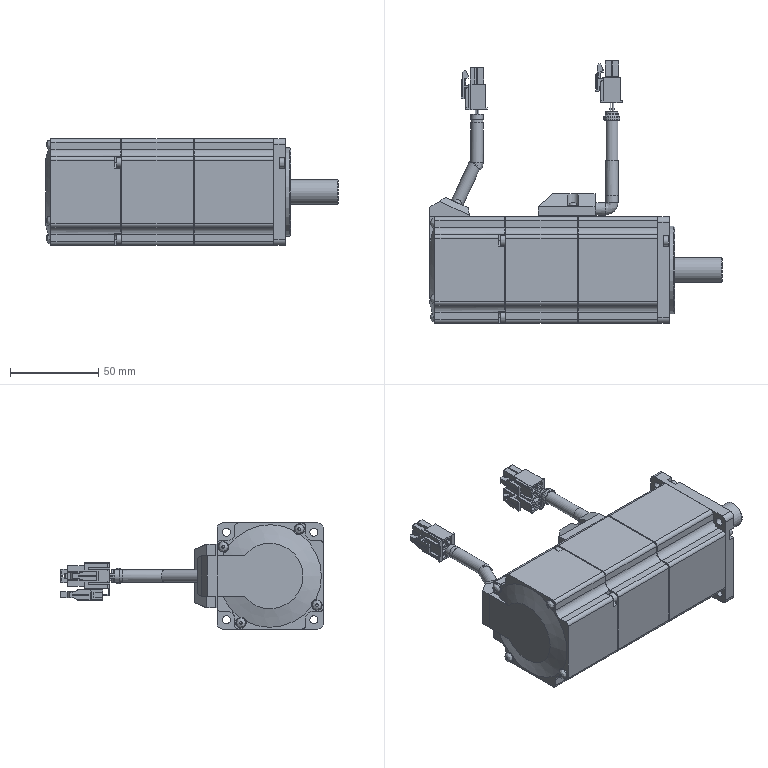Part | NX | 8 solids | 782 faces | box 165.5 x 148.3 x 60 mm | volume 467767 mm3 | plane 573 | cylinder 179 | spline 17 | cone 13 | commonest cylinder face diameters 4 x46 8 x24 0.6 x18 1 x16 2.6 x12 6.5 x12